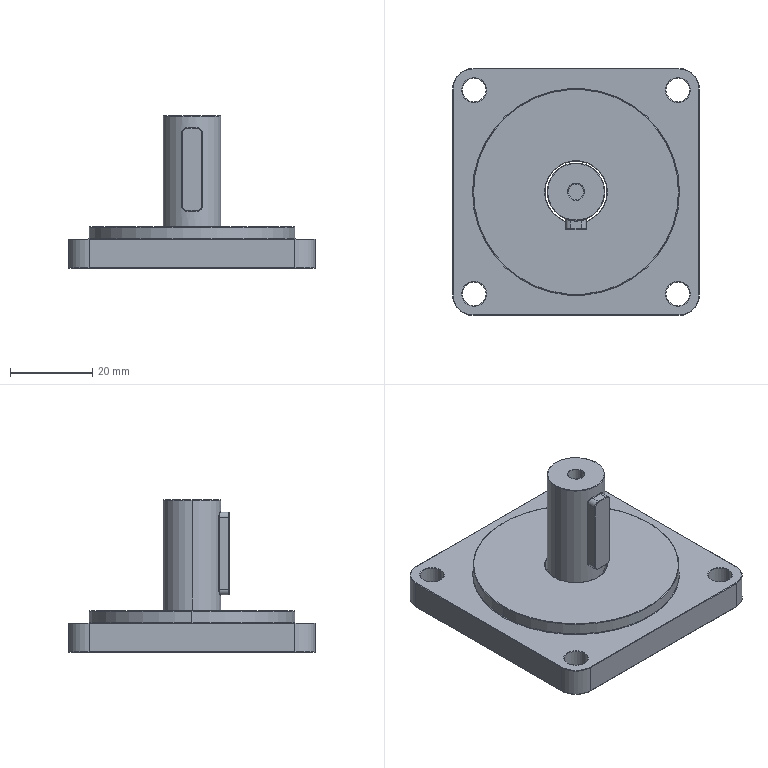Part | STEP file | HF-KE23B | 2 solids | 101 faces | box 60 x 60 x 37.084 mm | volume 33182 mm3 | torus 44 | cylinder 38 | plane 15 | spline 4 | commonest cylinder face diameters 0.254 x14 5.8 x8 2.54 x4 10 x4 4 x2 14 x2